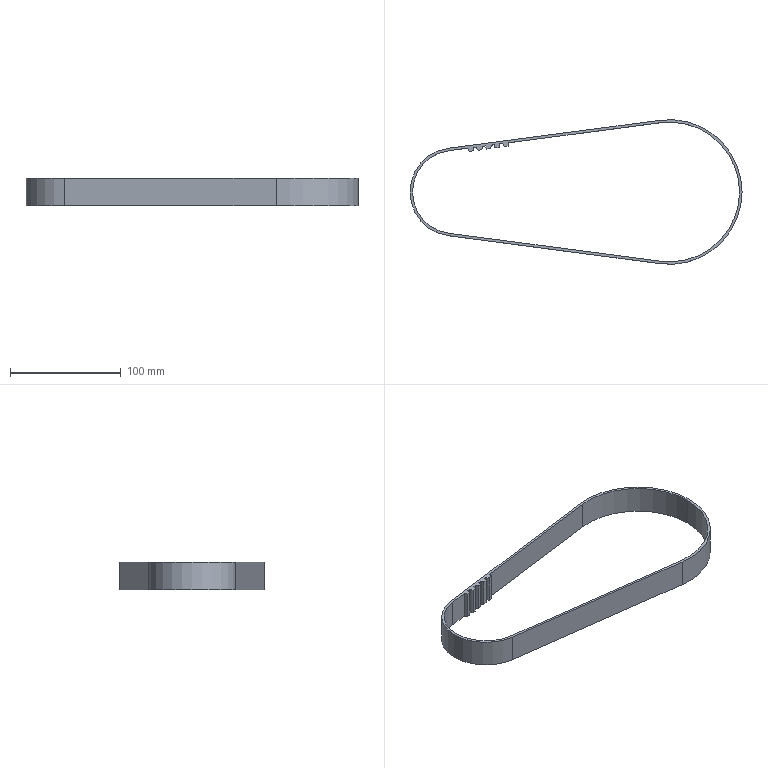Part | SolidWorks | features BaseBody 1 | 1 solid | 37 faces | box 299.317 x 130.452 x 25 mm | volume 41947 mm3 | cylinder 21 | plane 16 | commonest cylinder face diameters 10.4 x15 125.952 x2 130.452 x2 75.022 x1 79.522 x1
STEP:
#1=CARTESIAN_POINT('',(185.783,-64.664,-12.5));
#2=VERTEX_POINT('',#1);
#3=CARTESIAN_POINT('',(259.556,0.,-12.5));
#4=VERTEX_POINT('',#3);
#5=CARTESIAN_POINT('',(194.33,0.,-12.5));
#6=DIRECTION('',(0.,0.,1.));
#7=DIRECTION('',(1.,0.,0.));
#8=AXIS2_PLACEMENT_3D('',#5,#6,#7);
#9=CIRCLE('',#8,65.226);
#10=EDGE_CURVE('',#2,#4,#9,.T.);
#11=ORIENTED_EDGE('',*,*,#10,.T.);
#12=CARTESIAN_POINT('',(259.556,0.,12.5));
#13=VERTEX_POINT('',#12);
#14=CARTESIAN_POINT('',(259.556,0.,12.5));
#15=DIRECTION('',(0.,0.,1.));
#16=VECTOR('',#15,1000.);
#17=LINE('',#14,#16);
#18=EDGE_CURVE('',#4,#13,#17,.T.);
#19=ORIENTED_EDGE('',*,*,#18,.T.);
#20=CARTESIAN_POINT('',(185.783,-64.664,12.5));
#21=VERTEX_POINT('',#20);
#22=CARTESIAN_POINT('',(194.33,0.,12.5));
#23=DIRECTION('',(0.,0.,-1.));
#24=DIRECTION('',(1.,0.,0.));
#25=AXIS2_PLACEMENT_3D('',#22,#23,#24);
#26=CIRCLE('',#25,65.226);
#27=EDGE_CURVE('',#13,#21,#26,.T.);
#28=ORIENTED_EDGE('',*,*,#27,.T.);
#29=CARTESIAN_POINT('',(185.783,-64.664,12.5));
#30=DIRECTION('',(0.,0.,-1.));
#31=VECTOR('',#30,1000.);
#32=LINE('',#29,#31);
#33=EDGE_CURVE('',#21,#2,#32,.T.);
#34=ORIENTED_EDGE('',*,*,#33,.T.);
#35=EDGE_LOOP('',(#11,#19,#28,#34));
#36=FACE_OUTER_BOUND('',#35,.T.);
#37=CARTESIAN_POINT('',(194.33,0.,12.5));
#38=DIRECTION('',(0.,0.,1.));
#39=DIRECTION('',(1.,0.,0.));
#40=AXIS2_PLACEMENT_3D('',#37,#38,#39);
#41=CYLINDRICAL_SURFACE('',#40,65.226);
#42=ADVANCED_FACE('',(#36),#41,.T.);
#43=CARTESIAN_POINT('',(186.078,62.433,-12.5));
#44=VERTEX_POINT('',#43);
#45=CARTESIAN_POINT('',(257.306,0.,-12.5));
#46=VERTEX_POINT('',#45);
#47=CARTESIAN_POINT('',(194.33,0.,-12.5));
#48=DIRECTION('',(0.,0.,-1.));
#49=DIRECTION('',(1.,0.,0.));
#50=AXIS2_PLACEMENT_3D('',#47,#48,#49);
#51=CIRCLE('',#50,62.976);
#52=EDGE_CURVE('',#44,#46,#51,.T.);
#53=ORIENTED_EDGE('',*,*,#52,.T.);
#54=CARTESIAN_POINT('',(257.306,0.,12.5));
#55=VERTEX_POINT('',#54);
#56=CARTESIAN_POINT('',(257.306,0.,12.5));
#57=DIRECTION('',(0.,0.,1.));
#58=VECTOR('',#57,1000.);
#59=LINE('',#56,#58);
#60=EDGE_CURVE('',#46,#55,#59,.T.);
#61=ORIENTED_EDGE('',*,*,#60,.T.);
#62=CARTESIAN_POINT('',(186.078,62.433,12.5));
#63=VERTEX_POINT('',#62);
#64=CARTESIAN_POINT('',(194.33,0.,12.5));
#65=DIRECTION('',(0.,0.,-1.));
#66=DIRECTION('',(1.,0.,0.));
#67=AXIS2_PLACEMENT_3D('',#64,#65,#66);
#68=CIRCLE('',#67,62.976);
#69=EDGE_CURVE('',#63,#55,#68,.T.);
#70=ORIENTED_EDGE('',*,*,#69,.F.);
#71=CARTESIAN_POINT('',(186.078,62.433,12.5));
#72=DIRECTION('',(0.,0.,1.));
#73=VECTOR('',#72,1000.);
#74=LINE('',#71,#73);
#75=EDGE_CURVE('',#44,#63,#74,.T.);
#76=ORIENTED_EDGE('',*,*,#75,.F.);
#77=EDGE_LOOP('',(#53,#61,#70,#76));
#78=FACE_OUTER_BOUND('',#77,.T.);
#79=CARTESIAN_POINT('',(194.33,0.,12.5));
#80=DIRECTION('',(0.,0.,1.));
#81=DIRECTION('',(1.,0.,0.));
#82=AXIS2_PLACEMENT_3D('',#79,#80,#81);
#83=CYLINDRICAL_SURFACE('',#82,62.976);
#84=ADVANCED_FACE('',(#78),#83,.F.);
#85=CARTESIAN_POINT('',(48.634,41.189,-12.5));
#86=VERTEX_POINT('',#85);
#87=CARTESIAN_POINT('',(49.259,43.661,-12.5));
#88=VERTEX_POINT('',#87);
#89=CARTESIAN_POINT('',(44.059,43.661,-12.5));
#90=DIRECTION('',(0.,0.,1.));
#91=DIRECTION('',(1.,0.,0.));
#92=AXIS2_PLACEMENT_3D('',#89,#90,#91);
#93=CIRCLE('',#92,5.2);
#94=EDGE_CURVE('',#86,#88,#93,.T.);
#95=ORIENTED_EDGE('',*,*,#94,.T.);
#96=CARTESIAN_POINT('',(49.259,43.661,12.5));
#97=VERTEX_POINT('',#96);
#98=CARTESIAN_POINT('',(49.259,43.661,12.5));
#99=DIRECTION('',(0.,0.,1.));
#100=VECTOR('',#99,1000.);
#101=LINE('',#98,#100);
#102=EDGE_CURVE('',#88,#97,#101,.T.);
#103=ORIENTED_EDGE('',*,*,#102,.T.);
#104=CARTESIAN_POINT('',(48.634,41.189,12.5));
#105=VERTEX_POINT('',#104);
#106=CARTESIAN_POINT('',(44.059,43.661,12.5));
#107=DIRECTION('',(0.,0.,1.));
#108=DIRECTION('',(1.,0.,0.));
#109=AXIS2_PLACEMENT_3D('',#106,#107,#108);
#110=CIRCLE('',#109,5.2);
#111=EDGE_CURVE('',#105,#97,#110,.T.);
#112=ORIENTED_EDGE('',*,*,#111,.F.);
#113=CARTESIAN_POINT('',(48.634,41.189,12.5));
#114=DIRECTION('',(0.,0.,-1.));
#115=VECTOR('',#114,1000.);
#116=LINE('',#113,#115);
#117=EDGE_CURVE('',#105,#86,#116,.T.);
#118=ORIENTED_EDGE('',*,*,#117,.T.);
#119=EDGE_LOOP('',(#95,#103,#112,#118));
#120=FACE_OUTER_BOUND('',#119,.T.);
#121=CARTESIAN_POINT('',(44.059,43.661,12.5));
#122=DIRECTION('',(0.,0.,1.));
#123=DIRECTION('',(1.,0.,0.));
#124=AXIS2_PLACEMENT_3D('',#121,#122,#123);
#125=CYLINDRICAL_SURFACE('',#124,5.2);
#126=ADVANCED_FACE('',(#120),#125,.T.);
#127=CARTESIAN_POINT('',(40.703,40.141,-12.5));
#128=VERTEX_POINT('',#127);
#129=CARTESIAN_POINT('',(41.328,42.613,-12.5));
#130=VERTEX_POINT('',#129);
#131=CARTESIAN_POINT('',(36.128,42.613,-12.5));
#132=DIRECTION('',(0.,0.,1.));
#133=DIRECTION('',(1.,0.,0.));
#134=AXIS2_PLACEMENT_3D('',#131,#132,#133);
#135=CIRCLE('',#134,5.2);
#136=EDGE_CURVE('',#128,#130,#135,.T.);
#137=ORIENTED_EDGE('',*,*,#136,.T.);
#138=CARTESIAN_POINT('',(41.328,42.613,12.5));
#139=VERTEX_POINT('',#138);
#140=CARTESIAN_POINT('',(41.328,42.613,12.5));
#141=DIRECTION('',(0.,0.,1.));
#142=VECTOR('',#141,1000.);
#143=LINE('',#140,#142);
#144=EDGE_CURVE('',#130,#139,#143,.T.);
#145=ORIENTED_EDGE('',*,*,#144,.T.);
#146=CARTESIAN_POINT('',(40.703,40.141,12.5));
#147=VERTEX_POINT('',#146);
#148=CARTESIAN_POINT('',(36.128,42.613,12.5));
#149=DIRECTION('',(0.,0.,1.));
#150=DIRECTION('',(1.,0.,0.));
#151=AXIS2_PLACEMENT_3D('',#148,#149,#150);
#152=CIRCLE('',#151,5.2);
#153=EDGE_CURVE('',#147,#139,#152,.T.);
#154=ORIENTED_EDGE('',*,*,#153,.F.);
#155=CARTESIAN_POINT('',(40.703,40.141,12.5));
#156=DIRECTION('',(0.,0.,-1.));
#157=VECTOR('',#156,1000.);
#158=LINE('',#155,#157);
#159=EDGE_CURVE('',#147,#128,#158,.T.);
#160=ORIENTED_EDGE('',*,*,#159,.T.);
#161=EDGE_LOOP('',(#137,#145,#154,#160));
#162=FACE_OUTER_BOUND('',#161,.T.);
#163=CARTESIAN_POINT('',(36.128,42.613,12.5));
#164=DIRECTION('',(0.,0.,1.));
#165=DIRECTION('',(1.,0.,0.));
#166=AXIS2_PLACEMENT_3D('',#163,#164,#165);
#167=CYLINDRICAL_SURFACE('',#166,5.2);
#168=ADVANCED_FACE('',(#162),#167,.T.);
#169=CARTESIAN_POINT('',(32.772,39.093,-12.5));
#170=VERTEX_POINT('',#169);
#171=CARTESIAN_POINT('',(33.397,41.564,-12.5));
#172=VERTEX_POINT('',#171);
#173=CARTESIAN_POINT('',(28.197,41.564,-12.5));
#174=DIRECTION('',(0.,0.,1.));
#175=DIRECTION('',(1.,0.,0.));
#176=AXIS2_PLACEMENT_3D('',#173,#174,#175);
#177=CIRCLE('',#176,5.2);
#178=EDGE_CURVE('',#170,#172,#177,.T.);
#179=ORIENTED_EDGE('',*,*,#178,.T.);
#180=CARTESIAN_POINT('',(33.397,41.564,12.5));
#181=VERTEX_POINT('',#180);
#182=CARTESIAN_POINT('',(33.397,41.564,12.5));
#183=DIRECTION('',(0.,0.,1.));
#184=VECTOR('',#183,1000.);
#185=LINE('',#182,#184);
#186=EDGE_CURVE('',#172,#181,#185,.T.);
#187=ORIENTED_EDGE('',*,*,#186,.T.);
#188=CARTESIAN_POINT('',(32.772,39.093,12.5));
#189=VERTEX_POINT('',#188);
#190=CARTESIAN_POINT('',(28.197,41.564,12.5));
#191=DIRECTION('',(0.,0.,1.));
#192=DIRECTION('',(1.,0.,0.));
#193=AXIS2_PLACEMENT_3D('',#190,#191,#192);
#194=CIRCLE('',#193,5.2);
#195=EDGE_CURVE('',#189,#181,#194,.T.);
#196=ORIENTED_EDGE('',*,*,#195,.F.);
#197=CARTESIAN_POINT('',(32.772,39.093,12.5));
#198=DIRECTION('',(0.,0.,-1.));
#199=VECTOR('',#198,1000.);
#200=LINE('',#197,#199);
#201=EDGE_CURVE('',#189,#170,#200,.T.);
#202=ORIENTED_EDGE('',*,*,#201,.T.);
#203=EDGE_LOOP('',(#179,#187,#196,#202));
#204=FACE_OUTER_BOUND('',#203,.T.);
#205=CARTESIAN_POINT('',(28.197,41.564,12.5));
#206=DIRECTION('',(0.,0.,1.));
#207=DIRECTION('',(1.,0.,0.));
#208=AXIS2_PLACEMENT_3D('',#205,#206,#207);
#209=CYLINDRICAL_SURFACE('',#208,5.2);
#210=ADVANCED_FACE('',(#204),#209,.T.);
#211=CARTESIAN_POINT('',(24.841,38.044,-12.5));
#212=VERTEX_POINT('',#211);
#213=CARTESIAN_POINT('',(25.466,40.516,-12.5));
#214=VERTEX_POINT('',#213);
#215=CARTESIAN_POINT('',(20.266,40.516,-12.5));
#216=DIRECTION('',(0.,0.,1.));
#217=DIRECTION('',(1.,0.,0.));
#218=AXIS2_PLACEMENT_3D('',#215,#216,#217);
#219=CIRCLE('',#218,5.2);
#220=EDGE_CURVE('',#212,#214,#219,.T.);
#221=ORIENTED_EDGE('',*,*,#220,.T.);
#222=CARTESIAN_POINT('',(25.466,40.516,12.5));
#223=VERTEX_POINT('',#222);
#224=CARTESIAN_POINT('',(25.466,40.516,12.5));
#225=DIRECTION('',(0.,0.,1.));
#226=VECTOR('',#225,1000.);
#227=LINE('',#224,#226);
#228=EDGE_CURVE('',#214,#223,#227,.T.);
#229=ORIENTED_EDGE('',*,*,#228,.T.);
#230=CARTESIAN_POINT('',(24.841,38.044,12.5));
#231=VERTEX_POINT('',#230);
#232=CARTESIAN_POINT('',(20.266,40.516,12.5));
#233=DIRECTION('',(0.,0.,1.));
#234=DIRECTION('',(1.,0.,0.));
#235=AXIS2_PLACEMENT_3D('',#232,#233,#234);
#236=CIRCLE('',#235,5.2);
#237=EDGE_CURVE('',#231,#223,#236,.T.);
#238=ORIENTED_EDGE('',*,*,#237,.F.);
#239=CARTESIAN_POINT('',(24.841,38.044,12.5));
#240=DIRECTION('',(0.,0.,-1.));
#241=VECTOR('',#240,1000.);
#242=LINE('',#239,#241);
#243=EDGE_CURVE('',#231,#212,#242,.T.);
#244=ORIENTED_EDGE('',*,*,#243,.T.);
#245=EDGE_LOOP('',(#221,#229,#238,#244));
#246=FACE_OUTER_BOUND('',#245,.T.);
#247=CARTESIAN_POINT('',(20.266,40.516,12.5));
#248=DIRECTION('',(0.,0.,1.));
#249=DIRECTION('',(1.,0.,0.));
#250=AXIS2_PLACEMENT_3D('',#247,#248,#249);
#251=CYLINDRICAL_SURFACE('',#250,5.2);
#252=ADVANCED_FACE('',(#246),#251,.T.);
#253=CARTESIAN_POINT('',(16.909,36.996,-12.5));
#254=VERTEX_POINT('',#253);
#255=CARTESIAN_POINT('',(17.535,39.468,-12.5));
#256=VERTEX_POINT('',#255);
#257=CARTESIAN_POINT('',(12.335,39.468,-12.5));
#258=DIRECTION('',(0.,0.,1.));
#259=DIRECTION('',(1.,0.,0.));
#260=AXIS2_PLACEMENT_3D('',#257,#258,#259);
#261=CIRCLE('',#260,5.2);
#262=EDGE_CURVE('',#254,#256,#261,.T.);
#263=ORIENTED_EDGE('',*,*,#262,.T.);
#264=CARTESIAN_POINT('',(17.535,39.468,12.5));
#265=VERTEX_POINT('',#264);
#266=CARTESIAN_POINT('',(17.535,39.468,12.5));
#267=DIRECTION('',(0.,0.,1.));
#268=VECTOR('',#267,1000.);
#269=LINE('',#266,#268);
#270=EDGE_CURVE('',#256,#265,#269,.T.);
#271=ORIENTED_EDGE('',*,*,#270,.T.);
#272=CARTESIAN_POINT('',(16.909,36.996,12.5));
#273=VERTEX_POINT('',#272);
#274=CARTESIAN_POINT('',(12.335,39.468,12.5));
#275=DIRECTION('',(0.,0.,1.));
#276=DIRECTION('',(1.,0.,0.));
#277=AXIS2_PLACEMENT_3D('',#274,#275,#276);
#278=CIRCLE('',#277,5.2);
#279=EDGE_CURVE('',#273,#265,#278,.T.);
#280=ORIENTED_EDGE('',*,*,#279,.F.);
#281=CARTESIAN_POINT('',(16.909,36.996,12.5));
#282=DIRECTION('',(0.,0.,-1.));
#283=VECTOR('',#282,1000.);
#284=LINE('',#281,#283);
#285=EDGE_CURVE('',#273,#254,#284,.T.);
#286=ORIENTED_EDGE('',*,*,#285,.T.);
#287=EDGE_LOOP('',(#263,#271,#280,#286));
#288=FACE_OUTER_BOUND('',#287,.T.);
#289=CARTESIAN_POINT('',(12.335,39.468,12.5));
#290=DIRECTION('',(0.,0.,1.));
#291=DIRECTION('',(1.,0.,0.));
#292=AXIS2_PLACEMENT_3D('',#289,#290,#291);
#293=CYLINDRICAL_SURFACE('',#292,5.2);
#294=ADVANCED_FACE('',(#288),#293,.T.);
#295=ORIENTED_EDGE('',*,*,#18,.F.);
#296=CARTESIAN_POINT('',(185.783,64.664,-12.5));
#297=VERTEX_POINT('',#296);
#298=CARTESIAN_POINT('',(194.33,0.,-12.5));
#299=DIRECTION('',(0.,0.,1.));
#300=DIRECTION('',(1.,0.,0.));
#301=AXIS2_PLACEMENT_3D('',#298,#299,#300);
#302=CIRCLE('',#301,65.226);
#303=EDGE_CURVE('',#4,#297,#302,.T.);
#304=ORIENTED_EDGE('',*,*,#303,.T.);
#305=CARTESIAN_POINT('',(185.783,64.664,12.5));
#306=VERTEX_POINT('',#305);
#307=CARTESIAN_POINT('',(185.783,64.664,12.5));
#308=DIRECTION('',(0.,0.,1.));
#309=VECTOR('',#308,1000.);
#310=LINE('',#307,#309);
#311=EDGE_CURVE('',#297,#306,#310,.T.);
#312=ORIENTED_EDGE('',*,*,#311,.T.);
#313=CARTESIAN_POINT('',(194.33,0.,12.5));
#314=DIRECTION('',(0.,0.,-1.));
#315=DIRECTION('',(1.,0.,0.));
#316=AXIS2_PLACEMENT_3D('',#313,#314,#315);
#317=CIRCLE('',#316,65.226);
#318=EDGE_CURVE('',#306,#13,#317,.T.);
#319=ORIENTED_EDGE('',*,*,#318,.T.);
#320=EDGE_LOOP('',(#295,#304,#312,#319));
#321=FACE_OUTER_BOUND('',#320,.T.);
#322=CARTESIAN_POINT('',(194.33,0.,12.5));
#323=DIRECTION('',(0.,0.,1.));
#324=DIRECTION('',(1.,0.,0.));
#325=AXIS2_PLACEMENT_3D('',#322,#323,#324);
#326=CYLINDRICAL_SURFACE('',#325,65.226);
#327=ADVANCED_FACE('',(#321),#326,.T.);
#328=ORIENTED_EDGE('',*,*,#33,.F.);
#329=CARTESIAN_POINT('',(-5.21,-39.418,12.5));
#330=VERTEX_POINT('',#329);
#331=CARTESIAN_POINT('',(-5.21,-39.418,12.5));
#332=DIRECTION('',(0.9914,-0.131,0.));
#333=VECTOR('',#332,1000.);
#334=LINE('',#331,#333);
#335=EDGE_CURVE('',#330,#21,#334,.T.);
#336=ORIENTED_EDGE('',*,*,#335,.F.);
#337=CARTESIAN_POINT('',(-5.21,-39.418,-12.5));
#338=VERTEX_POINT('',#337);
#339=CARTESIAN_POINT('',(-5.21,-39.418,12.5));
#340=DIRECTION('',(0.,0.,1.));
#341=VECTOR('',#340,1000.);
#342=LINE('',#339,#341);
#343=EDGE_CURVE('',#338,#330,#342,.T.);
#344=ORIENTED_EDGE('',*,*,#343,.F.);
#345=CARTESIAN_POINT('',(-5.21,-39.418,-12.5));
#346=DIRECTION('',(-0.9914,0.131,0.));
#347=VECTOR('',#346,1000.);
#348=LINE('',#345,#347);
#349=EDGE_CURVE('',#2,#338,#348,.T.);
#350=ORIENTED_EDGE('',*,*,#349,.F.);
#351=EDGE_LOOP('',(#328,#336,#344,#350));
#352=FACE_OUTER_BOUND('',#351,.T.);
#353=CARTESIAN_POINT('',(-5.21,-39.418,12.5));
#354=DIRECTION('',(0.131,0.9914,0.));
#355=DIRECTION('',(-0.9914,0.131,0.));
#356=AXIS2_PLACEMENT_3D('',#353,#354,#355);
#357=PLANE('',#356);
#358=ADVANCED_FACE('',(#352),#357,.F.);
#359=CARTESIAN_POINT('',(186.078,-62.433,12.5));
#360=VERTEX_POINT('',#359);
#361=CARTESIAN_POINT('',(-4.915,-37.188,12.5));
#362=VERTEX_POINT('',#361);
#363=CARTESIAN_POINT('',(186.078,-62.433,12.5));
#364=DIRECTION('',(-0.9914,0.131,0.));
#365=VECTOR('',#364,1000.);
#366=LINE('',#363,#365);
#367=EDGE_CURVE('',#360,#362,#366,.T.);
#368=ORIENTED_EDGE('',*,*,#367,.T.);
#369=CARTESIAN_POINT('',(-4.915,37.188,12.5));
#370=VERTEX_POINT('',#369);
#371=CARTESIAN_POINT('',(0.,0.,12.5));
#372=DIRECTION('',(0.,0.,-1.));
#373=DIRECTION('',(1.,0.,0.));
#374=AXIS2_PLACEMENT_3D('',#371,#372,#373);
#375=CIRCLE('',#374,37.511);
#376=EDGE_CURVE('',#362,#370,#375,.T.);
#377=ORIENTED_EDGE('',*,*,#376,.T.);
#378=CARTESIAN_POINT('',(12.335,39.468,12.5));
#379=VERTEX_POINT('',#378);
#380=CARTESIAN_POINT('',(-4.915,37.188,12.5));
#381=DIRECTION('',(0.9914,0.131,0.));
#382=VECTOR('',#381,1000.);
#383=LINE('',#380,#382);
#384=EDGE_CURVE('',#370,#379,#383,.T.);
#385=ORIENTED_EDGE('',*,*,#384,.T.);
#386=CARTESIAN_POINT('',(13.714,36.574,12.5));
#387=VERTEX_POINT('',#386);
#388=CARTESIAN_POINT('',(17.49,40.149,12.5));
#389=DIRECTION('',(0.,0.,1.));
#390=DIRECTION('',(1.,0.,0.));
#391=AXIS2_PLACEMENT_3D('',#388,#389,#390);
#392=CIRCLE('',#391,5.2);
#393=EDGE_CURVE('',#379,#387,#392,.T.);
#394=ORIENTED_EDGE('',*,*,#393,.T.);
#395=CARTESIAN_POINT('',(13.714,36.574,12.5));
#396=DIRECTION('',(0.9914,0.131,0.));
#397=VECTOR('',#396,1000.);
#398=LINE('',#395,#397);
#399=EDGE_CURVE('',#387,#273,#398,.T.);
#400=ORIENTED_EDGE('',*,*,#399,.T.);
#401=ORIENTED_EDGE('',*,*,#279,.T.);
#402=CARTESIAN_POINT('',(17.49,40.149,12.5));
#403=VERTEX_POINT('',#402);
#404=CARTESIAN_POINT('',(12.335,39.468,12.5));
#405=DIRECTION('',(0.,0.,1.));
#406=DIRECTION('',(1.,0.,0.));
#407=AXIS2_PLACEMENT_3D('',#404,#405,#406);
#408=CIRCLE('',#407,5.2);
#409=EDGE_CURVE('',#265,#403,#408,.T.);
#410=ORIENTED_EDGE('',*,*,#409,.T.);
#411=CARTESIAN_POINT('',(20.266,40.516,12.5));
#412=VERTEX_POINT('',#411);
#413=CARTESIAN_POINT('',(17.49,40.149,12.5));
#414=DIRECTION('',(0.9914,0.131,0.));
#415=VECTOR('',#414,1000.);
#416=LINE('',#413,#415);
#417=EDGE_CURVE('',#403,#412,#416,.T.);
#418=ORIENTED_EDGE('',*,*,#417,.T.);
#419=CARTESIAN_POINT('',(21.645,37.622,12.5));
#420=VERTEX_POINT('',#419);
#421=CARTESIAN_POINT('',(25.421,41.198,12.5));
#422=DIRECTION('',(0.,0.,1.));
#423=DIRECTION('',(1.,0.,0.));
#424=AXIS2_PLACEMENT_3D('',#421,#422,#423);
#425=CIRCLE('',#424,5.2);
#426=EDGE_CURVE('',#412,#420,#425,.T.);
#427=ORIENTED_EDGE('',*,*,#426,.T.);
#428=CARTESIAN_POINT('',(21.645,37.622,12.5));
#429=DIRECTION('',(0.9914,0.131,0.));
#430=VECTOR('',#429,1000.);
#431=LINE('',#428,#430);
#432=EDGE_CURVE('',#420,#231,#431,.T.);
#433=ORIENTED_EDGE('',*,*,#432,.T.);
#434=ORIENTED_EDGE('',*,*,#237,.T.);
#435=CARTESIAN_POINT('',(25.421,41.198,12.5));
#436=VERTEX_POINT('',#435);
#437=CARTESIAN_POINT('',(20.266,40.516,12.5));
#438=DIRECTION('',(0.,0.,1.));
#439=DIRECTION('',(1.,0.,0.));
#440=AXIS2_PLACEMENT_3D('',#437,#438,#439);
#441=CIRCLE('',#440,5.2);
#442=EDGE_CURVE('',#223,#436,#441,.T.);
#443=ORIENTED_EDGE('',*,*,#442,.T.);
#444=CARTESIAN_POINT('',(28.197,41.564,12.5));
#445=VERTEX_POINT('',#444);
#446=CARTESIAN_POINT('',(25.421,41.198,12.5));
#447=DIRECTION('',(0.9914,0.131,0.));
#448=VECTOR('',#447,1000.);
#449=LINE('',#446,#448);
#450=EDGE_CURVE('',#436,#445,#449,.T.);
#451=ORIENTED_EDGE('',*,*,#450,.T.);
#452=CARTESIAN_POINT('',(29.576,38.67,12.5));
#453=VERTEX_POINT('',#452);
#454=CARTESIAN_POINT('',(33.352,42.246,12.5));
#455=DIRECTION('',(0.,0.,1.));
#456=DIRECTION('',(1.,0.,0.));
#457=AXIS2_PLACEMENT_3D('',#454,#455,#456);
#458=CIRCLE('',#457,5.2);
#459=EDGE_CURVE('',#445,#453,#458,.T.);
#460=ORIENTED_EDGE('',*,*,#459,.T.);
#461=CARTESIAN_POINT('',(29.576,38.67,12.5));
#462=DIRECTION('',(0.9914,0.131,0.));
#463=VECTOR('',#462,1000.);
#464=LINE('',#461,#463);
#465=EDGE_CURVE('',#453,#189,#464,.T.);
#466=ORIENTED_EDGE('',*,*,#465,.T.);
#467=ORIENTED_EDGE('',*,*,#195,.T.);
#468=CARTESIAN_POINT('',(33.352,42.246,12.5));
#469=VERTEX_POINT('',#468);
#470=CARTESIAN_POINT('',(28.197,41.564,12.5));
#471=DIRECTION('',(0.,0.,1.));
#472=DIRECTION('',(1.,0.,0.));
#473=AXIS2_PLACEMENT_3D('',#470,#471,#472);
#474=CIRCLE('',#473,5.2);
#475=EDGE_CURVE('',#181,#469,#474,.T.);
#476=ORIENTED_EDGE('',*,*,#475,.T.);
#477=CARTESIAN_POINT('',(36.128,42.613,12.5));
#478=VERTEX_POINT('',#477);
#479=CARTESIAN_POINT('',(33.352,42.246,12.5));
#480=DIRECTION('',(0.9914,0.131,0.));
#481=VECTOR('',#480,1000.);
#482=LINE('',#479,#481);
#483=EDGE_CURVE('',#469,#478,#482,.T.);
#484=ORIENTED_EDGE('',*,*,#483,.T.);
#485=CARTESIAN_POINT('',(37.507,39.719,12.5));
#486=VERTEX_POINT('',#485);
#487=CARTESIAN_POINT('',(41.283,43.294,12.5));
#488=DIRECTION('',(0.,0.,1.));
#489=DIRECTION('',(1.,0.,0.));
#490=AXIS2_PLACEMENT_3D('',#487,#488,#489);
#491=CIRCLE('',#490,5.2);
#492=EDGE_CURVE('',#478,#486,#491,.T.);
#493=ORIENTED_EDGE('',*,*,#492,.T.);
#494=CARTESIAN_POINT('',(37.507,39.719,12.5));
#495=DIRECTION('',(0.9914,0.131,0.));
#496=VECTOR('',#495,1000.);
#497=LINE('',#494,#496);
#498=EDGE_CURVE('',#486,#147,#497,.T.);
#499=ORIENTED_EDGE('',*,*,#498,.T.);
#500=ORIENTED_EDGE('',*,*,#153,.T.);
#501=CARTESIAN_POINT('',(41.283,43.294,12.5));
#502=VERTEX_POINT('',#501);
#503=CARTESIAN_POINT('',(36.128,42.613,12.5));
#504=DIRECTION('',(0.,0.,1.));
#505=DIRECTION('',(1.,0.,0.));
#506=AXIS2_PLACEMENT_3D('',#503,#504,#505);
#507=CIRCLE('',#506,5.2);
#508=EDGE_CURVE('',#139,#502,#507,.T.);
#509=ORIENTED_EDGE('',*,*,#508,.T.);
#510=CARTESIAN_POINT('',(44.059,43.661,12.5));
#511=VERTEX_POINT('',#510);
#512=CARTESIAN_POINT('',(41.283,43.294,12.5));
#513=DIRECTION('',(0.9914,0.131,0.));
#514=VECTOR('',#513,1000.);
#515=LINE('',#512,#514);
#516=EDGE_CURVE('',#502,#511,#515,.T.);
#517=ORIENTED_EDGE('',*,*,#516,.T.);
#518=CARTESIAN_POINT('',(45.438,40.767,12.5));
#519=VERTEX_POINT('',#518);
#520=CARTESIAN_POINT('',(49.214,44.342,12.5));
#521=DIRECTION('',(0.,0.,1.));
#522=DIRECTION('',(1.,0.,0.));
#523=AXIS2_PLACEMENT_3D('',#520,#521,#522);
#524=CIRCLE('',#523,5.2);
#525=EDGE_CURVE('',#511,#519,#524,.T.);
#526=ORIENTED_EDGE('',*,*,#525,.T.);
#527=CARTESIAN_POINT('',(45.438,40.767,12.5));
#528=DIRECTION('',(0.9914,0.131,0.));
#529=VECTOR('',#528,1000.);
#530=LINE('',#527,#529);
#531=EDGE_CURVE('',#519,#105,#530,.T.);
#532=ORIENTED_EDGE('',*,*,#531,.T.);
#533=ORIENTED_EDGE('',*,*,#111,.T.);
#534=CARTESIAN_POINT('',(49.214,44.342,12.5));
#535=VERTEX_POINT('',#534);
#536=CARTESIAN_POINT('',(44.059,43.661,12.5));
#537=DIRECTION('',(0.,0.,1.));
#538=DIRECTION('',(1.,0.,0.));
#539=AXIS2_PLACEMENT_3D('',#536,#537,#538);
#540=CIRCLE('',#539,5.2);
#541=EDGE_CURVE('',#97,#535,#540,.T.);
#542=ORIENTED_EDGE('',*,*,#541,.T.);
#543=CARTESIAN_POINT('',(49.214,44.342,12.5));
#544=DIRECTION('',(0.9914,0.131,0.));
#545=VECTOR('',#544,1000.);
#546=LINE('',#543,#545);
#547=EDGE_CURVE('',#535,#63,#546,.T.);
#548=ORIENTED_EDGE('',*,*,#547,.T.);
#549=ORIENTED_EDGE('',*,*,#69,.T.);
#550=CARTESIAN_POINT('',(194.33,0.,12.5));
#551=DIRECTION('',(0.,0.,-1.));
#552=DIRECTION('',(1.,0.,0.));
#553=AXIS2_PLACEMENT_3D('',#550,#551,#552);
#554=CIRCLE('',#553,62.976);
#555=EDGE_CURVE('',#55,#360,#554,.T.);
#556=ORIENTED_EDGE('',*,*,#555,.T.);
#557=EDGE_LOOP('',(#368,#377,#385,#394,#400,#401,#410,#418,#427,#433,#434,#443,#451,#460,#466,#467,#476,#484,#493,#499,#500,#509,#517,#526,#532,#533,#542,#548,#549,#556));
#558=FACE_BOUND('',#557,.T.);
#559=ORIENTED_EDGE('',*,*,#335,.T.);
#560=ORIENTED_EDGE('',*,*,#27,.F.);
#561=ORIENTED_EDGE('',*,*,#318,.F.);
#562=CARTESIAN_POINT('',(-5.21,39.418,12.5));
#563=VERTEX_POINT('',#562);
#564=CARTESIAN_POINT('',(185.783,64.664,12.5));
#565=DIRECTION('',(-0.9914,-0.131,0.));
#566=VECTOR('',#565,1000.);
#567=LINE('',#564,#566);
#568=EDGE_CURVE('',#306,#563,#567,.T.);
#569=ORIENTED_EDGE('',*,*,#568,.T.);
#570=CARTESIAN_POINT('',(0.,0.,12.5));
#571=DIRECTION('',(0.,0.,1.));
#572=DIRECTION('',(1.,0.,0.));
#573=AXIS2_PLACEMENT_3D('',#570,#571,#572);
#574=CIRCLE('',#573,39.761);
#575=EDGE_CURVE('',#563,#330,#574,.T.);
#576=ORIENTED_EDGE('',*,*,#575,.T.);
#577=EDGE_LOOP('',(#559,#560,#561,#569,#576));
#578=FACE_OUTER_BOUND('',#577,.T.);
#579=CARTESIAN_POINT('',(17.49,40.149,12.5));
#580=DIRECTION('',(0.,0.,1.));
#581=DIRECTION('',(1.,0.,0.));
#582=AXIS2_PLACEMENT_3D('',#579,#580,#581);
#583=PLANE('',#582);
#584=ADVANCED_FACE('',(#558,#578),#583,.T.);
#585=CARTESIAN_POINT('',(-5.21,39.418,-12.5));
#586=VERTEX_POINT('',#585);
#587=CARTESIAN_POINT('',(-5.21,39.418,12.5));
#588=DIRECTION('',(0.,0.,-1.));
#589=VECTOR('',#588,1000.);
#590=LINE('',#587,#589);
#591=EDGE_CURVE('',#563,#586,#590,.T.);
#592=ORIENTED_EDGE('',*,*,#591,.F.);
#593=ORIENTED_EDGE('',*,*,#568,.F.);
#594=ORIENTED_EDGE('',*,*,#311,.F.);
#595=CARTESIAN_POINT('',(50.307,46.757,-12.5));
#596=DIRECTION('',(0.9914,0.131,0.));
#597=VECTOR('',#596,1000.);
#598=LINE('',#595,#597);
#599=EDGE_CURVE('',#586,#297,#598,.T.);
#600=ORIENTED_EDGE('',*,*,#599,.F.);
#601=EDGE_LOOP('',(#592,#593,#594,#600));
#602=FACE_OUTER_BOUND('',#601,.T.);
#603=CARTESIAN_POINT('',(50.307,46.757,12.5));
#604=DIRECTION('',(0.131,-0.9914,0.));
#605=DIRECTION('',(0.9914,0.131,0.));
#606=AXIS2_PLACEMENT_3D('',#603,#604,#605);
#607=PLANE('',#606);
#608=ADVANCED_FACE('',(#602),#607,.F.);
#609=CARTESIAN_POINT('',(-4.915,-37.188,-12.5));
#610=VERTEX_POINT('',#609);
#611=CARTESIAN_POINT('',(-4.915,37.188,-12.5));
#612=VERTEX_POINT('',#611);
#613=CARTESIAN_POINT('',(0.,0.,-12.5));
#614=DIRECTION('',(0.,0.,-1.));
#615=DIRECTION('',(1.,0.,0.));
#616=AXIS2_PLACEMENT_3D('',#613,#614,#615);
#617=CIRCLE('',#616,37.511);
#618=EDGE_CURVE('',#610,#612,#617,.T.);
#619=ORIENTED_EDGE('',*,*,#618,.F.);
#620=CARTESIAN_POINT('',(186.078,-62.433,-12.5));
#621=VERTEX_POINT('',#620);
#622=CARTESIAN_POINT('',(186.078,-62.433,-12.5));
#623=DIRECTION('',(-0.9914,0.131,0.));
#624=VECTOR('',#623,1000.);
#625=LINE('',#622,#624);
#626=EDGE_CURVE('',#621,#610,#625,.T.);
#627=ORIENTED_EDGE('',*,*,#626,.F.);
#628=CARTESIAN_POINT('',(194.33,0.,-12.5));
#629=DIRECTION('',(0.,0.,-1.));
#630=DIRECTION('',(1.,0.,0.));
#631=AXIS2_PLACEMENT_3D('',#628,#629,#630);
#632=CIRCLE('',#631,62.976);
#633=EDGE_CURVE('',#46,#621,#632,.T.);
#634=ORIENTED_EDGE('',*,*,#633,.F.);
#635=ORIENTED_EDGE('',*,*,#52,.F.);
#636=CARTESIAN_POINT('',(49.214,44.342,-12.5));
#637=VERTEX_POINT('',#636);
#638=CARTESIAN_POINT('',(49.214,44.342,-12.5));
#639=DIRECTION('',(0.9914,0.131,0.));
#640=VECTOR('',#639,1000.);
#641=LINE('',#638,#640);
#642=EDGE_CURVE('',#637,#44,#641,.T.);
#643=ORIENTED_EDGE('',*,*,#642,.F.);
#644=CARTESIAN_POINT('',(44.059,43.661,-12.5));
#645=DIRECTION('',(0.,0.,1.));
#646=DIRECTION('',(1.,0.,0.));
#647=AXIS2_PLACEMENT_3D('',#644,#645,#646);
#648=CIRCLE('',#647,5.2);
#649=EDGE_CURVE('',#88,#637,#648,.T.);
#650=ORIENTED_EDGE('',*,*,#649,.F.);
#651=ORIENTED_EDGE('',*,*,#94,.F.);
#652=CARTESIAN_POINT('',(45.438,40.767,-12.5));
#653=VERTEX_POINT('',#652);
#654=CARTESIAN_POINT('',(45.438,40.767,-12.5));
#655=DIRECTION('',(0.9914,0.131,0.));
#656=VECTOR('',#655,1000.);
#657=LINE('',#654,#656);
#658=EDGE_CURVE('',#653,#86,#657,.T.);
#659=ORIENTED_EDGE('',*,*,#658,.F.);
#660=CARTESIAN_POINT('',(44.059,43.661,-12.5));
#661=VERTEX_POINT('',#660);
#662=CARTESIAN_POINT('',(49.214,44.342,-12.5));
#663=DIRECTION('',(0.,0.,1.));
#664=DIRECTION('',(1.,0.,0.));
#665=AXIS2_PLACEMENT_3D('',#662,#663,#664);
#666=CIRCLE('',#665,5.2);
#667=EDGE_CURVE('',#661,#653,#666,.T.);
#668=ORIENTED_EDGE('',*,*,#667,.F.);
#669=CARTESIAN_POINT('',(41.283,43.294,-12.5));
#670=VERTEX_POINT('',#669);
#671=CARTESIAN_POINT('',(41.283,43.294,-12.5));
#672=DIRECTION('',(0.9914,0.131,0.));
#673=VECTOR('',#672,1000.);
#674=LINE('',#671,#673);
#675=EDGE_CURVE('',#670,#661,#674,.T.);
#676=ORIENTED_EDGE('',*,*,#675,.F.);
#677=CARTESIAN_POINT('',(36.128,42.613,-12.5));
#678=DIRECTION('',(0.,0.,1.));
#679=DIRECTION('',(1.,0.,0.));
#680=AXIS2_PLACEMENT_3D('',#677,#678,#679);
#681=CIRCLE('',#680,5.2);
#682=EDGE_CURVE('',#130,#670,#681,.T.);
#683=ORIENTED_EDGE('',*,*,#682,.F.);
#684=ORIENTED_EDGE('',*,*,#136,.F.);
#685=CARTESIAN_POINT('',(37.507,39.719,-12.5));
#686=VERTEX_POINT('',#685);
#687=CARTESIAN_POINT('',(37.507,39.719,-12.5));
#688=DIRECTION('',(0.9914,0.131,0.));
#689=VECTOR('',#688,1000.);
#690=LINE('',#687,#689);
#691=EDGE_CURVE('',#686,#128,#690,.T.);
#692=ORIENTED_EDGE('',*,*,#691,.F.);
#693=CARTESIAN_POINT('',(36.128,42.613,-12.5));
#694=VERTEX_POINT('',#693);
#695=CARTESIAN_POINT('',(41.283,43.294,-12.5));
#696=DIRECTION('',(0.,0.,1.));
#697=DIRECTION('',(1.,0.,0.));
#698=AXIS2_PLACEMENT_3D('',#695,#696,#697);
#699=CIRCLE('',#698,5.2);
#700=EDGE_CURVE('',#694,#686,#699,.T.);
#701=ORIENTED_EDGE('',*,*,#700,.F.);
#702=CARTESIAN_POINT('',(33.352,42.246,-12.5));
#703=VERTEX_POINT('',#702);
#704=CARTESIAN_POINT('',(33.352,42.246,-12.5));
#705=DIRECTION('',(0.9914,0.131,0.));
#706=VECTOR('',#705,1000.);
#707=LINE('',#704,#706);
#708=EDGE_CURVE('',#703,#694,#707,.T.);
#709=ORIENTED_EDGE('',*,*,#708,.F.);
#710=CARTESIAN_POINT('',(28.197,41.564,-12.5));
#711=DIRECTION('',(0.,0.,1.));
#712=DIRECTION('',(1.,0.,0.));
#713=AXIS2_PLACEMENT_3D('',#710,#711,#712);
#714=CIRCLE('',#713,5.2);
#715=EDGE_CURVE('',#172,#703,#714,.T.);
#716=ORIENTED_EDGE('',*,*,#715,.F.);
#717=ORIENTED_EDGE('',*,*,#178,.F.);
#718=CARTESIAN_POINT('',(29.576,38.67,-12.5));
#719=VERTEX_POINT('',#718);
#720=CARTESIAN_POINT('',(29.576,38.67,-12.5));
#721=DIRECTION('',(0.9914,0.131,0.));
#722=VECTOR('',#721,1000.);
#723=LINE('',#720,#722);
#724=EDGE_CURVE('',#719,#170,#723,.T.);
#725=ORIENTED_EDGE('',*,*,#724,.F.);
#726=CARTESIAN_POINT('',(28.197,41.564,-12.5));
#727=VERTEX_POINT('',#726);
#728=CARTESIAN_POINT('',(33.352,42.246,-12.5));
#729=DIRECTION('',(0.,0.,1.));
#730=DIRECTION('',(1.,0.,0.));
#731=AXIS2_PLACEMENT_3D('',#728,#729,#730);
#732=CIRCLE('',#731,5.2);
#733=EDGE_CURVE('',#727,#719,#732,.T.);
#734=ORIENTED_EDGE('',*,*,#733,.F.);
#735=CARTESIAN_POINT('',(25.421,41.198,-12.5));
#736=VERTEX_POINT('',#735);
#737=CARTESIAN_POINT('',(25.421,41.198,-12.5));
#738=DIRECTION('',(0.9914,0.131,0.));
#739=VECTOR('',#738,1000.);
#740=LINE('',#737,#739);
#741=EDGE_CURVE('',#736,#727,#740,.T.);
#742=ORIENTED_EDGE('',*,*,#741,.F.);
#743=CARTESIAN_POINT('',(20.266,40.516,-12.5));
#744=DIRECTION('',(0.,0.,1.));
#745=DIRECTION('',(1.,0.,0.));
#746=AXIS2_PLACEMENT_3D('',#743,#744,#745);
#747=CIRCLE('',#746,5.2);
#748=EDGE_CURVE('',#214,#736,#747,.T.);
#749=ORIENTED_EDGE('',*,*,#748,.F.);
#750=ORIENTED_EDGE('',*,*,#220,.F.);
#751=CARTESIAN_POINT('',(21.645,37.622,-12.5));
#752=VERTEX_POINT('',#751);
#753=CARTESIAN_POINT('',(21.645,37.622,-12.5));
#754=DIRECTION('',(0.9914,0.131,0.));
#755=VECTOR('',#754,1000.);
#756=LINE('',#753,#755);
#757=EDGE_CURVE('',#752,#212,#756,.T.);
#758=ORIENTED_EDGE('',*,*,#757,.F.);
#759=CARTESIAN_POINT('',(20.266,40.516,-12.5));
#760=VERTEX_POINT('',#759);
#761=CARTESIAN_POINT('',(25.421,41.198,-12.5));
#762=DIRECTION('',(0.,0.,1.));
#763=DIRECTION('',(1.,0.,0.));
#764=AXIS2_PLACEMENT_3D('',#761,#762,#763);
#765=CIRCLE('',#764,5.2);
#766=EDGE_CURVE('',#760,#752,#765,.T.);
#767=ORIENTED_EDGE('',*,*,#766,.F.);
#768=CARTESIAN_POINT('',(17.49,40.149,-12.5));
#769=VERTEX_POINT('',#768);
#770=CARTESIAN_POINT('',(17.49,40.149,-12.5));
#771=DIRECTION('',(0.9914,0.131,0.));
#772=VECTOR('',#771,1000.);
#773=LINE('',#770,#772);
#774=EDGE_CURVE('',#769,#760,#773,.T.);
#775=ORIENTED_EDGE('',*,*,#774,.F.);
#776=CARTESIAN_POINT('',(12.335,39.468,-12.5));
#777=DIRECTION('',(0.,0.,1.));
#778=DIRECTION('',(1.,0.,0.));
#779=AXIS2_PLACEMENT_3D('',#776,#777,#778);
#780=CIRCLE('',#779,5.2);
#781=EDGE_CURVE('',#256,#769,#780,.T.);
#782=ORIENTED_EDGE('',*,*,#781,.F.);
#783=ORIENTED_EDGE('',*,*,#262,.F.);
#784=CARTESIAN_POINT('',(13.714,36.574,-12.5));
#785=VERTEX_POINT('',#784);
#786=CARTESIAN_POINT('',(13.714,36.574,-12.5));
#787=DIRECTION('',(0.9914,0.131,0.));
#788=VECTOR('',#787,1000.);
#789=LINE('',#786,#788);
#790=EDGE_CURVE('',#785,#254,#789,.T.);
#791=ORIENTED_EDGE('',*,*,#790,.F.);
#792=CARTESIAN_POINT('',(12.335,39.468,-12.5));
#793=VERTEX_POINT('',#792);
#794=CARTESIAN_POINT('',(17.49,40.149,-12.5));
#795=DIRECTION('',(0.,0.,1.));
#796=DIRECTION('',(1.,0.,0.));
#797=AXIS2_PLACEMENT_3D('',#794,#795,#796);
#798=CIRCLE('',#797,5.2);
#799=EDGE_CURVE('',#793,#785,#798,.T.);
#800=ORIENTED_EDGE('',*,*,#799,.F.);
#801=CARTESIAN_POINT('',(-4.915,37.188,-12.5));
#802=DIRECTION('',(0.9914,0.131,0.));
#803=VECTOR('',#802,1000.);
#804=LINE('',#801,#803);
#805=EDGE_CURVE('',#612,#793,#804,.T.);
#806=ORIENTED_EDGE('',*,*,#805,.F.);
#807=EDGE_LOOP('',(#619,#627,#634,#635,#643,#650,#651,#659,#668,#676,#683,#684,#692,#701,#709,#716,#717,#725,#734,#742,#749,#750,#758,#767,#775,#782,#783,#791,#800,#806));
#808=FACE_BOUND('',#807,.T.);
#809=ORIENTED_EDGE('',*,*,#599,.T.);
#810=ORIENTED_EDGE('',*,*,#303,.F.);
#811=ORIENTED_EDGE('',*,*,#10,.F.);
#812=ORIENTED_EDGE('',*,*,#349,.T.);
#813=CARTESIAN_POINT('',(0.,0.,-12.5));
#814=DIRECTION('',(0.,0.,1.));
#815=DIRECTION('',(1.,0.,0.));
#816=AXIS2_PLACEMENT_3D('',#813,#814,#815);
#817=CIRCLE('',#816,39.761);
#818=EDGE_CURVE('',#586,#338,#817,.T.);
#819=ORIENTED_EDGE('',*,*,#818,.F.);
#820=EDGE_LOOP('',(#809,#810,#811,#812,#819));
#821=FACE_OUTER_BOUND('',#820,.T.);
#822=CARTESIAN_POINT('',(17.49,40.149,-12.5));
#823=DIRECTION('',(0.,0.,1.));
#824=DIRECTION('',(1.,0.,0.));
#825=AXIS2_PLACEMENT_3D('',#822,#823,#824);
#826=PLANE('',#825);
#827=ADVANCED_FACE('',(#808,#821),#826,.F.);
#828=ORIENTED_EDGE('',*,*,#343,.T.);
#829=ORIENTED_EDGE('',*,*,#575,.F.);
#830=ORIENTED_EDGE('',*,*,#591,.T.);
#831=ORIENTED_EDGE('',*,*,#818,.T.);
#832=EDGE_LOOP('',(#828,#829,#830,#831));
#833=FACE_OUTER_BOUND('',#832,.T.);
#834=CARTESIAN_POINT('',(0.,0.,12.5));
#835=DIRECTION('',(0.,0.,1.));
#836=DIRECTION('',(1.,0.,0.));
#837=AXIS2_PLACEMENT_3D('',#834,#835,#836);
#838=CYLINDRICAL_SURFACE('',#837,39.761);
#839=ADVANCED_FACE('',(#833),#838,.T.);
#840=CARTESIAN_POINT('',(-4.915,-37.188,12.5));
#841=DIRECTION('',(0.,0.,1.));
#842=VECTOR('',#841,1000.);
#843=LINE('',#840,#842);
#844=EDGE_CURVE('',#610,#362,#843,.T.);
#845=ORIENTED_EDGE('',*,*,#844,.F.);
#846=ORIENTED_EDGE('',*,*,#618,.T.);
#847=CARTESIAN_POINT('',(-4.915,37.188,12.5));
#848=DIRECTION('',(0.,0.,1.));
#849=VECTOR('',#848,1000.);
#850=LINE('',#847,#849);
#851=EDGE_CURVE('',#612,#370,#850,.T.);
#852=ORIENTED_EDGE('',*,*,#851,.T.);
#853=ORIENTED_EDGE('',*,*,#376,.F.);
#854=EDGE_LOOP('',(#845,#846,#852,#853));
#855=FACE_OUTER_BOUND('',#854,.T.);
#856=CARTESIAN_POINT('',(0.,0.,12.5));
#857=DIRECTION('',(0.,0.,1.));
#858=DIRECTION('',(1.,0.,0.));
#859=AXIS2_PLACEMENT_3D('',#856,#857,#858);
#860=CYLINDRICAL_SURFACE('',#859,37.511);
#861=ADVANCED_FACE('',(#855),#860,.F.);
#862=ORIENTED_EDGE('',*,*,#367,.F.);
#863=CARTESIAN_POINT('',(186.078,-62.433,12.5));
#864=DIRECTION('',(0.,0.,-1.));
#865=VECTOR('',#864,1000.);
#866=LINE('',#863,#865);
#867=EDGE_CURVE('',#360,#621,#866,.T.);
#868=ORIENTED_EDGE('',*,*,#867,.T.);
#869=ORIENTED_EDGE('',*,*,#626,.T.);
#870=ORIENTED_EDGE('',*,*,#844,.T.);
#871=EDGE_LOOP('',(#862,#868,#869,#870));
#872=FACE_OUTER_BOUND('',#871,.T.);
#873=CARTESIAN_POINT('',(-4.915,-37.188,12.5));
#874=DIRECTION('',(0.131,0.9914,0.));
#875=DIRECTION('',(-0.9914,0.131,0.));
#876=AXIS2_PLACEMENT_3D('',#873,#874,#875);
#877=PLANE('',#876);
#878=ADVANCED_FACE('',(#872),#877,.T.);
#879=ORIENTED_EDGE('',*,*,#60,.F.);
#880=ORIENTED_EDGE('',*,*,#633,.T.);
#881=ORIENTED_EDGE('',*,*,#867,.F.);
#882=ORIENTED_EDGE('',*,*,#555,.F.);
#883=EDGE_LOOP('',(#879,#880,#881,#882));
#884=FACE_OUTER_BOUND('',#883,.T.);
#885=CARTESIAN_POINT('',(194.33,0.,12.5));
#886=DIRECTION('',(0.,0.,1.));
#887=DIRECTION('',(1.,0.,0.));
#888=AXIS2_PLACEMENT_3D('',#885,#886,#887);
#889=CYLINDRICAL_SURFACE('',#888,62.976);
#890=ADVANCED_FACE('',(#884),#889,.F.);
#891=ORIENTED_EDGE('',*,*,#75,.T.);
#892=ORIENTED_EDGE('',*,*,#547,.F.);
#893=CARTESIAN_POINT('',(49.214,44.342,12.5));
#894=DIRECTION('',(0.,0.,1.));
#895=VECTOR('',#894,1000.);
#896=LINE('',#893,#895);
#897=EDGE_CURVE('',#637,#535,#896,.T.);
#898=ORIENTED_EDGE('',*,*,#897,.F.);
#899=ORIENTED_EDGE('',*,*,#642,.T.);
#900=EDGE_LOOP('',(#891,#892,#898,#899));
#901=FACE_OUTER_BOUND('',#900,.T.);
#902=CARTESIAN_POINT('',(49.214,44.342,12.5));
#903=DIRECTION('',(-0.131,0.9914,0.));
#904=DIRECTION('',(-0.9914,-0.131,0.));
#905=AXIS2_PLACEMENT_3D('',#902,#903,#904);
#906=PLANE('',#905);
#907=ADVANCED_FACE('',(#901),#906,.F.);
#908=ORIENTED_EDGE('',*,*,#102,.F.);
#909=ORIENTED_EDGE('',*,*,#649,.T.);
#910=ORIENTED_EDGE('',*,*,#897,.T.);
#911=ORIENTED_EDGE('',*,*,#541,.F.);
#912=EDGE_LOOP('',(#908,#909,#910,#911));
#913=FACE_OUTER_BOUND('',#912,.T.);
#914=CARTESIAN_POINT('',(44.059,43.661,12.5));
#915=DIRECTION('',(0.,0.,1.));
#916=DIRECTION('',(1.,0.,0.));
#917=AXIS2_PLACEMENT_3D('',#914,#915,#916);
#918=CYLINDRICAL_SURFACE('',#917,5.2);
#919=ADVANCED_FACE('',(#913),#918,.T.);
#920=ORIENTED_EDGE('',*,*,#117,.F.);
#921=ORIENTED_EDGE('',*,*,#531,.F.);
#922=CARTESIAN_POINT('',(45.438,40.767,12.5));
#923=DIRECTION('',(0.,0.,1.));
#924=VECTOR('',#923,1000.);
#925=LINE('',#922,#924);
#926=EDGE_CURVE('',#653,#519,#925,.T.);
#927=ORIENTED_EDGE('',*,*,#926,.F.);
#928=ORIENTED_EDGE('',*,*,#658,.T.);
#929=EDGE_LOOP('',(#920,#921,#927,#928));
#930=FACE_OUTER_BOUND('',#929,.T.);
#931=CARTESIAN_POINT('',(45.438,40.767,12.5));
#932=DIRECTION('',(-0.131,0.9914,0.));
#933=DIRECTION('',(-0.9914,-0.131,0.));
#934=AXIS2_PLACEMENT_3D('',#931,#932,#933);
#935=PLANE('',#934);
#936=ADVANCED_FACE('',(#930),#935,.F.);
#937=ORIENTED_EDGE('',*,*,#525,.F.);
#938=CARTESIAN_POINT('',(44.059,43.661,12.5));
#939=DIRECTION('',(0.,0.,-1.));
#940=VECTOR('',#939,1000.);
#941=LINE('',#938,#940);
#942=EDGE_CURVE('',#511,#661,#941,.T.);
#943=ORIENTED_EDGE('',*,*,#942,.T.);
#944=ORIENTED_EDGE('',*,*,#667,.T.);
#945=ORIENTED_EDGE('',*,*,#926,.T.);
#946=EDGE_LOOP('',(#937,#943,#944,#945));
#947=FACE_OUTER_BOUND('',#946,.T.);
#948=CARTESIAN_POINT('',(49.214,44.342,12.5));
#949=DIRECTION('',(0.,0.,1.));
#950=DIRECTION('',(1.,0.,0.));
#951=AXIS2_PLACEMENT_3D('',#948,#949,#950);
#952=CYLINDRICAL_SURFACE('',#951,5.2);
#953=ADVANCED_FACE('',(#947),#952,.T.);
#954=ORIENTED_EDGE('',*,*,#942,.F.);
#955=ORIENTED_EDGE('',*,*,#516,.F.);
#956=CARTESIAN_POINT('',(41.283,43.294,12.5));
#957=DIRECTION('',(0.,0.,1.));
#958=VECTOR('',#957,1000.);
#959=LINE('',#956,#958);
#960=EDGE_CURVE('',#670,#502,#959,.T.);
#961=ORIENTED_EDGE('',*,*,#960,.F.);
#962=ORIENTED_EDGE('',*,*,#675,.T.);
#963=EDGE_LOOP('',(#954,#955,#961,#962));
#964=FACE_OUTER_BOUND('',#963,.T.);
#965=CARTESIAN_POINT('',(41.283,43.294,12.5));
#966=DIRECTION('',(-0.131,0.9914,0.));
#967=DIRECTION('',(-0.9914,-0.131,0.));
#968=AXIS2_PLACEMENT_3D('',#965,#966,#967);
#969=PLANE('',#968);
#970=ADVANCED_FACE('',(#964),#969,.F.);
#971=ORIENTED_EDGE('',*,*,#144,.F.);
#972=ORIENTED_EDGE('',*,*,#682,.T.);
#973=ORIENTED_EDGE('',*,*,#960,.T.);
#974=ORIENTED_EDGE('',*,*,#508,.F.);
#975=EDGE_LOOP('',(#971,#972,#973,#974));
#976=FACE_OUTER_BOUND('',#975,.T.);
#977=CARTESIAN_POINT('',(36.128,42.613,12.5));
#978=DIRECTION('',(0.,0.,1.));
#979=DIRECTION('',(1.,0.,0.));
#980=AXIS2_PLACEMENT_3D('',#977,#978,#979);
#981=CYLINDRICAL_SURFACE('',#980,5.2);
#982=ADVANCED_FACE('',(#976),#981,.T.);
#983=ORIENTED_EDGE('',*,*,#159,.F.);
#984=ORIENTED_EDGE('',*,*,#498,.F.);
#985=CARTESIAN_POINT('',(37.507,39.719,12.5));
#986=DIRECTION('',(0.,0.,1.));
#987=VECTOR('',#986,1000.);
#988=LINE('',#985,#987);
#989=EDGE_CURVE('',#686,#486,#988,.T.);
#990=ORIENTED_EDGE('',*,*,#989,.F.);
#991=ORIENTED_EDGE('',*,*,#691,.T.);
#992=EDGE_LOOP('',(#983,#984,#990,#991));
#993=FACE_OUTER_BOUND('',#992,.T.);
#994=CARTESIAN_POINT('',(37.507,39.719,12.5));
#995=DIRECTION('',(-0.131,0.9914,0.));
#996=DIRECTION('',(-0.9914,-0.131,0.));
#997=AXIS2_PLACEMENT_3D('',#994,#995,#996);
#998=PLANE('',#997);
#999=ADVANCED_FACE('',(#993),#998,.F.);
#1000=ORIENTED_EDGE('',*,*,#492,.F.);
#1001=CARTESIAN_POINT('',(36.128,42.613,12.5));
#1002=DIRECTION('',(0.,0.,-1.));
#1003=VECTOR('',#1002,1000.);
#1004=LINE('',#1001,#1003);
#1005=EDGE_CURVE('',#478,#694,#1004,.T.);
#1006=ORIENTED_EDGE('',*,*,#1005,.T.);
#1007=ORIENTED_EDGE('',*,*,#700,.T.);
#1008=ORIENTED_EDGE('',*,*,#989,.T.);
#1009=EDGE_LOOP('',(#1000,#1006,#1007,#1008));
#1010=FACE_OUTER_BOUND('',#1009,.T.);
#1011=CARTESIAN_POINT('',(41.283,43.294,12.5));
#1012=DIRECTION('',(0.,0.,1.));
#1013=DIRECTION('',(1.,0.,0.));
#1014=AXIS2_PLACEMENT_3D('',#1011,#1012,#1013);
#1015=CYLINDRICAL_SURFACE('',#1014,5.2);
#1016=ADVANCED_FACE('',(#1010),#1015,.T.);
#1017=ORIENTED_EDGE('',*,*,#1005,.F.);
#1018=ORIENTED_EDGE('',*,*,#483,.F.);
#1019=CARTESIAN_POINT('',(33.352,42.246,12.5));
#1020=DIRECTION('',(0.,0.,1.));
#1021=VECTOR('',#1020,1000.);
#1022=LINE('',#1019,#1021);
#1023=EDGE_CURVE('',#703,#469,#1022,.T.);
#1024=ORIENTED_EDGE('',*,*,#1023,.F.);
#1025=ORIENTED_EDGE('',*,*,#708,.T.);
#1026=EDGE_LOOP('',(#1017,#1018,#1024,#1025));
#1027=FACE_OUTER_BOUND('',#1026,.T.);
#1028=CARTESIAN_POINT('',(33.352,42.246,12.5));
#1029=DIRECTION('',(-0.131,0.9914,0.));
#1030=DIRECTION('',(-0.9914,-0.131,0.));
#1031=AXIS2_PLACEMENT_3D('',#1028,#1029,#1030);
#1032=PLANE('',#1031);
#1033=ADVANCED_FACE('',(#1027),#1032,.F.);
#1034=ORIENTED_EDGE('',*,*,#186,.F.);
#1035=ORIENTED_EDGE('',*,*,#715,.T.);
#1036=ORIENTED_EDGE('',*,*,#1023,.T.);
#1037=ORIENTED_EDGE('',*,*,#475,.F.);
#1038=EDGE_LOOP('',(#1034,#1035,#1036,#1037));
#1039=FACE_OUTER_BOUND('',#1038,.T.);
#1040=CARTESIAN_POINT('',(28.197,41.564,12.5));
#1041=DIRECTION('',(0.,0.,1.));
#1042=DIRECTION('',(1.,0.,0.));
#1043=AXIS2_PLACEMENT_3D('',#1040,#1041,#1042);
#1044=CYLINDRICAL_SURFACE('',#1043,5.2);
#1045=ADVANCED_FACE('',(#1039),#1044,.T.);
#1046=ORIENTED_EDGE('',*,*,#201,.F.);
#1047=ORIENTED_EDGE('',*,*,#465,.F.);
#1048=CARTESIAN_POINT('',(29.576,38.67,12.5));
#1049=DIRECTION('',(0.,0.,1.));
#1050=VECTOR('',#1049,1000.);
#1051=LINE('',#1048,#1050);
#1052=EDGE_CURVE('',#719,#453,#1051,.T.);
#1053=ORIENTED_EDGE('',*,*,#1052,.F.);
#1054=ORIENTED_EDGE('',*,*,#724,.T.);
#1055=EDGE_LOOP('',(#1046,#1047,#1053,#1054));
#1056=FACE_OUTER_BOUND('',#1055,.T.);
#1057=CARTESIAN_POINT('',(29.576,38.67,12.5));
#1058=DIRECTION('',(-0.131,0.9914,0.));
#1059=DIRECTION('',(-0.9914,-0.131,0.));
#1060=AXIS2_PLACEMENT_3D('',#1057,#1058,#1059);
#1061=PLANE('',#1060);
#1062=ADVANCED_FACE('',(#1056),#1061,.F.);
#1063=ORIENTED_EDGE('',*,*,#459,.F.);
#1064=CARTESIAN_POINT('',(28.197,41.564,12.5));
#1065=DIRECTION('',(0.,0.,-1.));
#1066=VECTOR('',#1065,1000.);
#1067=LINE('',#1064,#1066);
#1068=EDGE_CURVE('',#445,#727,#1067,.T.);
#1069=ORIENTED_EDGE('',*,*,#1068,.T.);
#1070=ORIENTED_EDGE('',*,*,#733,.T.);
#1071=ORIENTED_EDGE('',*,*,#1052,.T.);
#1072=EDGE_LOOP('',(#1063,#1069,#1070,#1071));
#1073=FACE_OUTER_BOUND('',#1072,.T.);
#1074=CARTESIAN_POINT('',(33.352,42.246,12.5));
#1075=DIRECTION('',(0.,0.,1.));
#1076=DIRECTION('',(1.,0.,0.));
#1077=AXIS2_PLACEMENT_3D('',#1074,#1075,#1076);
#1078=CYLINDRICAL_SURFACE('',#1077,5.2);
#1079=ADVANCED_FACE('',(#1073),#1078,.T.);
#1080=ORIENTED_EDGE('',*,*,#1068,.F.);
#1081=ORIENTED_EDGE('',*,*,#450,.F.);
#1082=CARTESIAN_POINT('',(25.421,41.198,12.5));
#1083=DIRECTION('',(0.,0.,1.));
#1084=VECTOR('',#1083,1000.);
#1085=LINE('',#1082,#1084);
#1086=EDGE_CURVE('',#736,#436,#1085,.T.);
#1087=ORIENTED_EDGE('',*,*,#1086,.F.);
#1088=ORIENTED_EDGE('',*,*,#741,.T.);
#1089=EDGE_LOOP('',(#1080,#1081,#1087,#1088));
#1090=FACE_OUTER_BOUND('',#1089,.T.);
#1091=CARTESIAN_POINT('',(25.421,41.198,12.5));
#1092=DIRECTION('',(-0.131,0.9914,0.));
#1093=DIRECTION('',(-0.9914,-0.131,0.));
#1094=AXIS2_PLACEMENT_3D('',#1091,#1092,#1093);
#1095=PLANE('',#1094);
#1096=ADVANCED_FACE('',(#1090),#1095,.F.);
#1097=ORIENTED_EDGE('',*,*,#228,.F.);
#1098=ORIENTED_EDGE('',*,*,#748,.T.);
#1099=ORIENTED_EDGE('',*,*,#1086,.T.);
#1100=ORIENTED_EDGE('',*,*,#442,.F.);
#1101=EDGE_LOOP('',(#1097,#1098,#1099,#1100));
#1102=FACE_OUTER_BOUND('',#1101,.T.);
#1103=CARTESIAN_POINT('',(20.266,40.516,12.5));
#1104=DIRECTION('',(0.,0.,1.));
#1105=DIRECTION('',(1.,0.,0.));
#1106=AXIS2_PLACEMENT_3D('',#1103,#1104,#1105);
#1107=CYLINDRICAL_SURFACE('',#1106,5.2);
#1108=ADVANCED_FACE('',(#1102),#1107,.T.);
#1109=ORIENTED_EDGE('',*,*,#243,.F.);
#1110=ORIENTED_EDGE('',*,*,#432,.F.);
#1111=CARTESIAN_POINT('',(21.645,37.622,12.5));
#1112=DIRECTION('',(0.,0.,1.));
#1113=VECTOR('',#1112,1000.);
#1114=LINE('',#1111,#1113);
#1115=EDGE_CURVE('',#752,#420,#1114,.T.);
#1116=ORIENTED_EDGE('',*,*,#1115,.F.);
#1117=ORIENTED_EDGE('',*,*,#757,.T.);
#1118=EDGE_LOOP('',(#1109,#1110,#1116,#1117));
#1119=FACE_OUTER_BOUND('',#1118,.T.);
#1120=CARTESIAN_POINT('',(21.645,37.622,12.5));
#1121=DIRECTION('',(-0.131,0.9914,0.));
#1122=DIRECTION('',(-0.9914,-0.131,0.));
#1123=AXIS2_PLACEMENT_3D('',#1120,#1121,#1122);
#1124=PLANE('',#1123);
#1125=ADVANCED_FACE('',(#1119),#1124,.F.);
#1126=ORIENTED_EDGE('',*,*,#426,.F.);
#1127=CARTESIAN_POINT('',(20.266,40.516,12.5));
#1128=DIRECTION('',(0.,0.,-1.));
#1129=VECTOR('',#1128,1000.);
#1130=LINE('',#1127,#1129);
#1131=EDGE_CURVE('',#412,#760,#1130,.T.);
#1132=ORIENTED_EDGE('',*,*,#1131,.T.);
#1133=ORIENTED_EDGE('',*,*,#766,.T.);
#1134=ORIENTED_EDGE('',*,*,#1115,.T.);
#1135=EDGE_LOOP('',(#1126,#1132,#1133,#1134));
#1136=FACE_OUTER_BOUND('',#1135,.T.);
#1137=CARTESIAN_POINT('',(25.421,41.198,12.5));
#1138=DIRECTION('',(0.,0.,1.));
#1139=DIRECTION('',(1.,0.,0.));
#1140=AXIS2_PLACEMENT_3D('',#1137,#1138,#1139);
#1141=CYLINDRICAL_SURFACE('',#1140,5.2);
#1142=ADVANCED_FACE('',(#1136),#1141,.T.);
#1143=ORIENTED_EDGE('',*,*,#1131,.F.);
#1144=ORIENTED_EDGE('',*,*,#417,.F.);
#1145=CARTESIAN_POINT('',(17.49,40.149,12.5));
#1146=DIRECTION('',(0.,0.,1.));
#1147=VECTOR('',#1146,1000.);
#1148=LINE('',#1145,#1147);
#1149=EDGE_CURVE('',#769,#403,#1148,.T.);
#1150=ORIENTED_EDGE('',*,*,#1149,.F.);
#1151=ORIENTED_EDGE('',*,*,#774,.T.);
#1152=EDGE_LOOP('',(#1143,#1144,#1150,#1151));
#1153=FACE_OUTER_BOUND('',#1152,.T.);
#1154=CARTESIAN_POINT('',(17.49,40.149,12.5));
#1155=DIRECTION('',(-0.131,0.9914,0.));
#1156=DIRECTION('',(-0.9914,-0.131,0.));
#1157=AXIS2_PLACEMENT_3D('',#1154,#1155,#1156);
#1158=PLANE('',#1157);
#1159=ADVANCED_FACE('',(#1153),#1158,.F.);
#1160=ORIENTED_EDGE('',*,*,#270,.F.);
#1161=ORIENTED_EDGE('',*,*,#781,.T.);
#1162=ORIENTED_EDGE('',*,*,#1149,.T.);
#1163=ORIENTED_EDGE('',*,*,#409,.F.);
#1164=EDGE_LOOP('',(#1160,#1161,#1162,#1163));
#1165=FACE_OUTER_BOUND('',#1164,.T.);
#1166=CARTESIAN_POINT('',(12.335,39.468,12.5));
#1167=DIRECTION('',(0.,0.,1.));
#1168=DIRECTION('',(1.,0.,0.));
#1169=AXIS2_PLACEMENT_3D('',#1166,#1167,#1168);
#1170=CYLINDRICAL_SURFACE('',#1169,5.2);
#1171=ADVANCED_FACE('',(#1165),#1170,.T.);
#1172=ORIENTED_EDGE('',*,*,#285,.F.);
#1173=ORIENTED_EDGE('',*,*,#399,.F.);
#1174=CARTESIAN_POINT('',(13.714,36.574,12.5));
#1175=DIRECTION('',(0.,0.,1.));
#1176=VECTOR('',#1175,1000.);
#1177=LINE('',#1174,#1176);
#1178=EDGE_CURVE('',#785,#387,#1177,.T.);
#1179=ORIENTED_EDGE('',*,*,#1178,.F.);
#1180=ORIENTED_EDGE('',*,*,#790,.T.);
#1181=EDGE_LOOP('',(#1172,#1173,#1179,#1180));
#1182=FACE_OUTER_BOUND('',#1181,.T.);
#1183=CARTESIAN_POINT('',(13.714,36.574,12.5));
#1184=DIRECTION('',(-0.131,0.9914,0.));
#1185=DIRECTION('',(-0.9914,-0.131,0.));
#1186=AXIS2_PLACEMENT_3D('',#1183,#1184,#1185);
#1187=PLANE('',#1186);
#1188=ADVANCED_FACE('',(#1182),#1187,.F.);
#1189=ORIENTED_EDGE('',*,*,#393,.F.);
#1190=CARTESIAN_POINT('',(12.335,39.468,12.5));
#1191=DIRECTION('',(0.,0.,-1.));
#1192=VECTOR('',#1191,1000.);
#1193=LINE('',#1190,#1192);
#1194=EDGE_CURVE('',#379,#793,#1193,.T.);
#1195=ORIENTED_EDGE('',*,*,#1194,.T.);
#1196=ORIENTED_EDGE('',*,*,#799,.T.);
#1197=ORIENTED_EDGE('',*,*,#1178,.T.);
#1198=EDGE_LOOP('',(#1189,#1195,#1196,#1197));
#1199=FACE_OUTER_BOUND('',#1198,.T.);
#1200=CARTESIAN_POINT('',(17.49,40.149,12.5));
#1201=DIRECTION('',(0.,0.,1.));
#1202=DIRECTION('',(1.,0.,0.));
#1203=AXIS2_PLACEMENT_3D('',#1200,#1201,#1202);
#1204=CYLINDRICAL_SURFACE('',#1203,5.2);
#1205=ADVANCED_FACE('',(#1199),#1204,.T.);
#1206=ORIENTED_EDGE('',*,*,#1194,.F.);
#1207=ORIENTED_EDGE('',*,*,#384,.F.);
#1208=ORIENTED_EDGE('',*,*,#851,.F.);
#1209=ORIENTED_EDGE('',*,*,#805,.T.);
#1210=EDGE_LOOP('',(#1206,#1207,#1208,#1209));
#1211=FACE_OUTER_BOUND('',#1210,.T.);
#1212=CARTESIAN_POINT('',(10.947,39.284,12.5));
#1213=DIRECTION('',(-0.131,0.9914,0.));
#1214=DIRECTION('',(-0.9914,-0.131,0.));
#1215=AXIS2_PLACEMENT_3D('',#1212,#1213,#1214);
#1216=PLANE('',#1215);
#1217=ADVANCED_FACE('',(#1211),#1216,.F.);
#1218=CLOSED_SHELL('',(#42,#84,#126,#168,#210,#252,#294,#327,#358,#584,#608,#827,#839,#861,#878,#890,#907,#919,#936,#953,#970,#982,#999,#1016,#1033,#1045,#1062,#1079,#1096,#1108,#1125,#1142,#1159,#1171,#1188,#1205,#1217));
#1219=MANIFOLD_SOLID_BREP('',#1218);
#1220=CARTESIAN_POINT('',(0.,0.,0.));
#1221=DIRECTION('',(0.,0.,1.));
#1222=DIRECTION('',(1.,0.,0.));
#1223=AXIS2_PLACEMENT_3D('',#1220,#1221,#1222);
#1224=(LENGTH_UNIT()NAMED_UNIT(*)SI_UNIT(.MILLI.,.METRE.));
#1225=UNCERTAINTY_MEASURE_WITH_UNIT(LENGTH_MEASURE(0.00001),#1224,'','');
#1226=(NAMED_UNIT(*)PLANE_ANGLE_UNIT()SI_UNIT($,.RADIAN.));
#1227=(NAMED_UNIT(*)SI_UNIT($,.STERADIAN.)SOLID_ANGLE_UNIT());
#1228=(GEOMETRIC_REPRESENTATION_CONTEXT(3)GLOBAL_UNCERTAINTY_ASSIGNED_CONTEXT((#1225))GLOBAL_UNIT_ASSIGNED_CONTEXT((#1224,#1226,#1227))REPRESENTATION_CONTEXT('',''));
#1229=ADVANCED_BREP_SHAPE_REPRESENTATION('',(#1219,#1223),#1228);